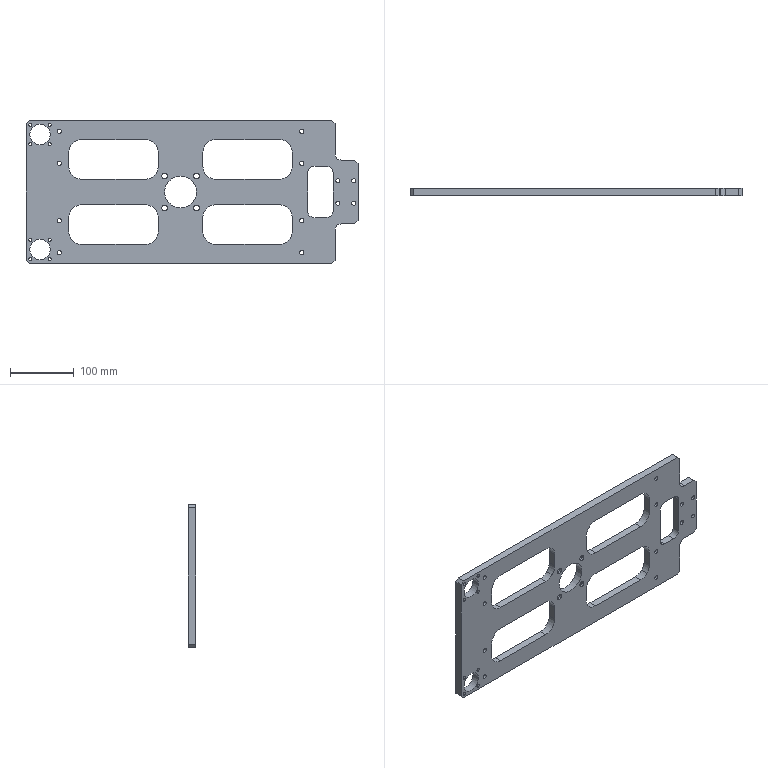Part | STEP file | CYL.MOUNT..stp | 1 solid | 172 faces | box 520 x 12 x 224 mm | volume 845705 mm3 | cylinder 84 | spline 50 | plane 38 | commonest cylinder face diameters 6.6 x16 11 x16 40 x16 5 x8 9 x8 14 x8